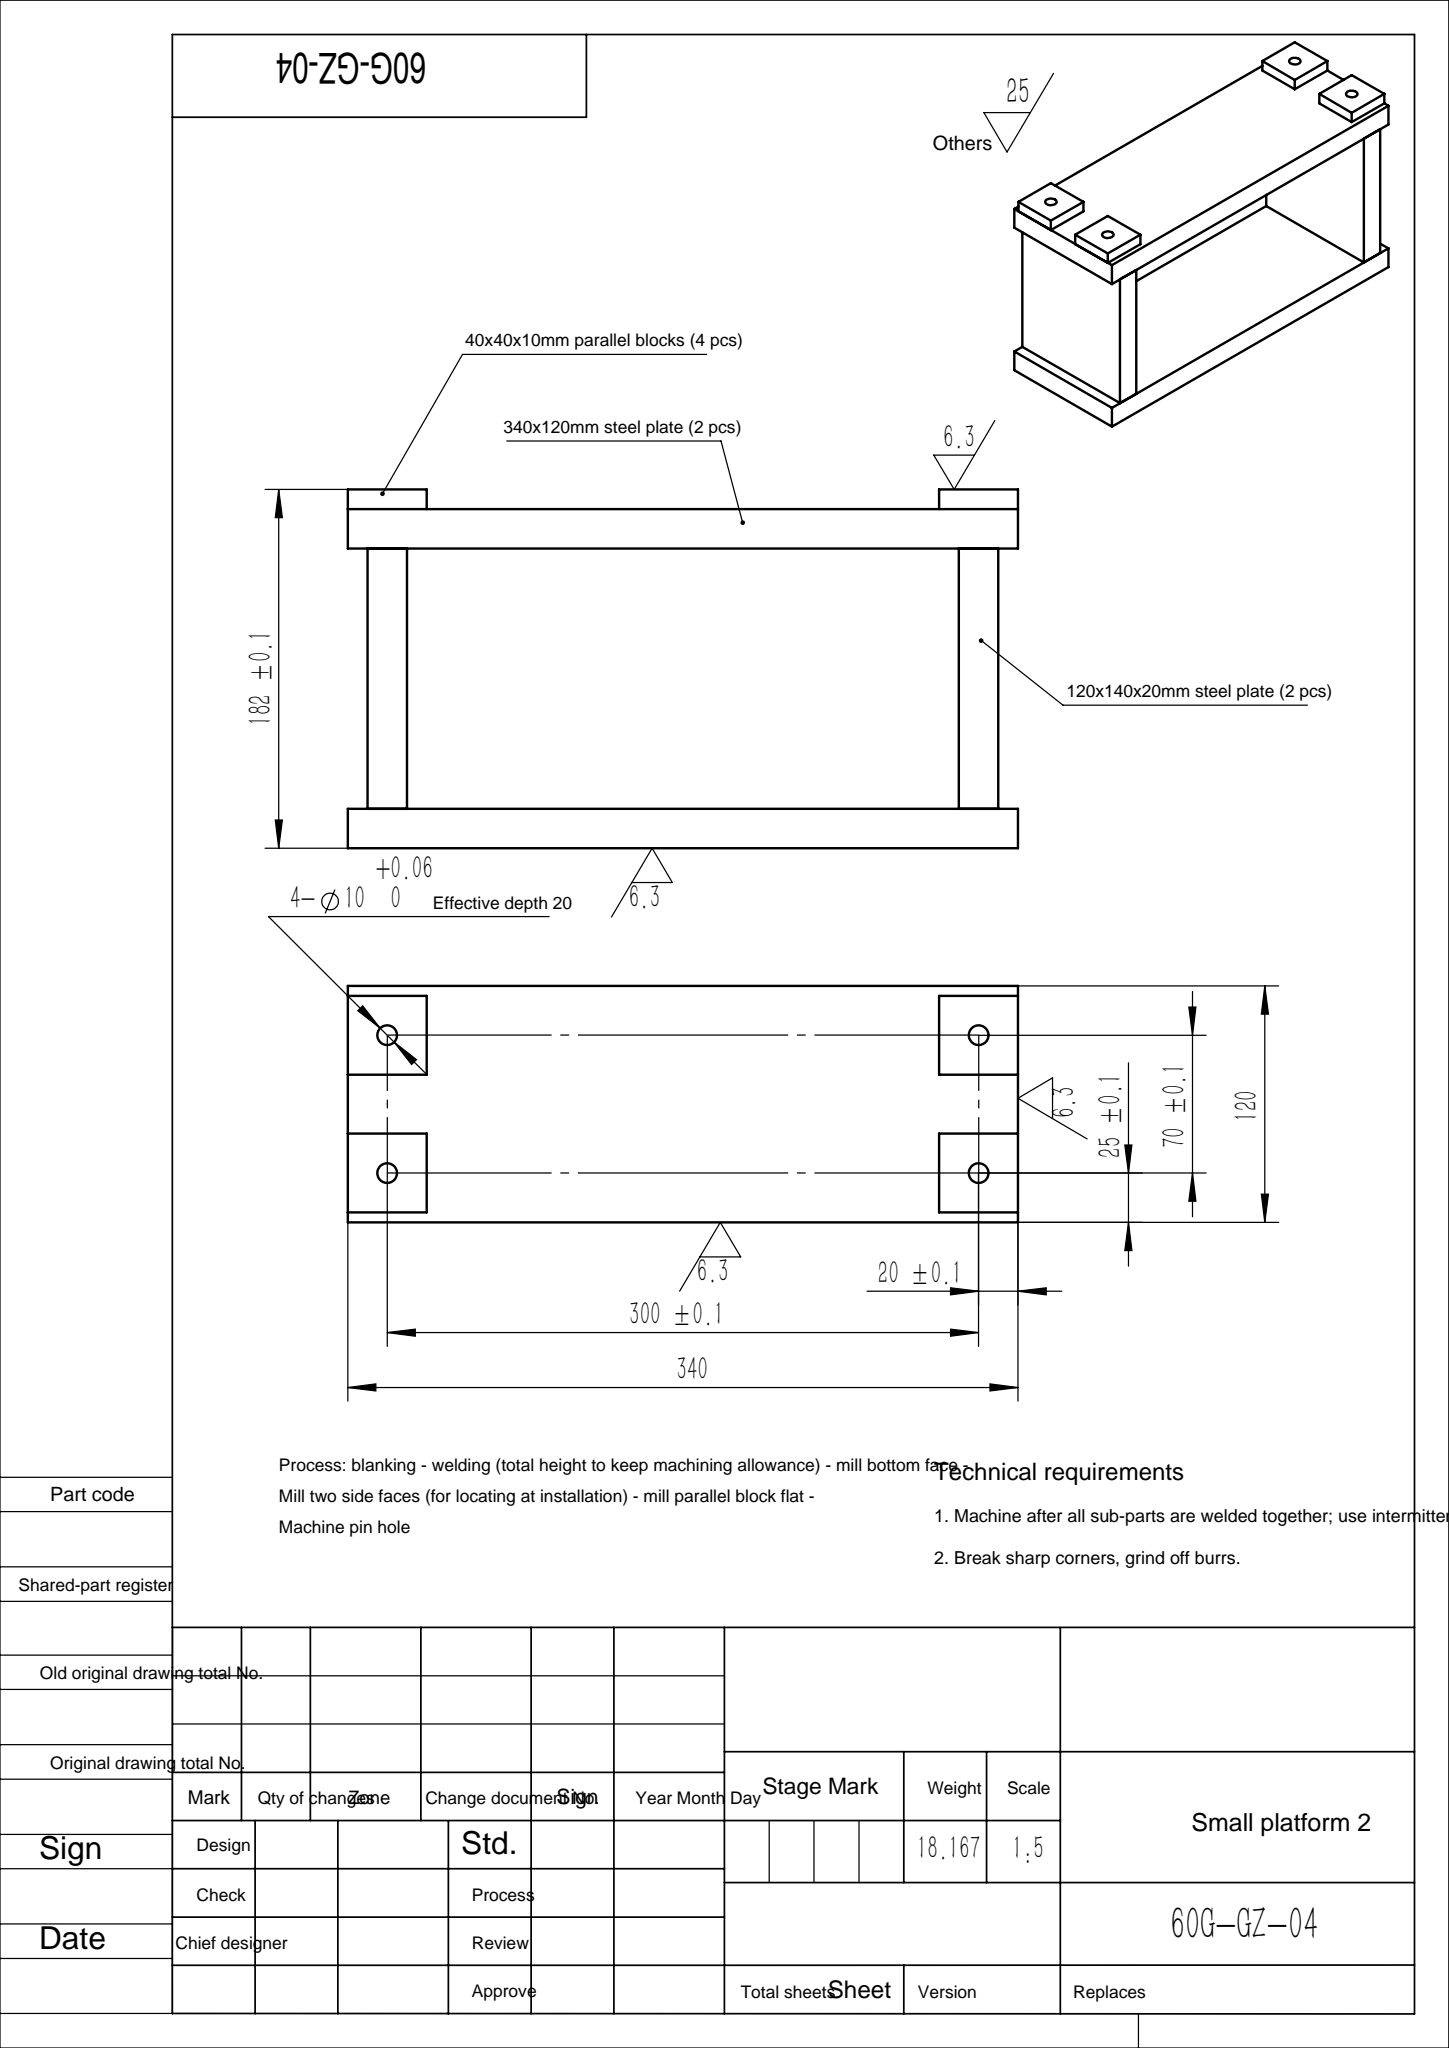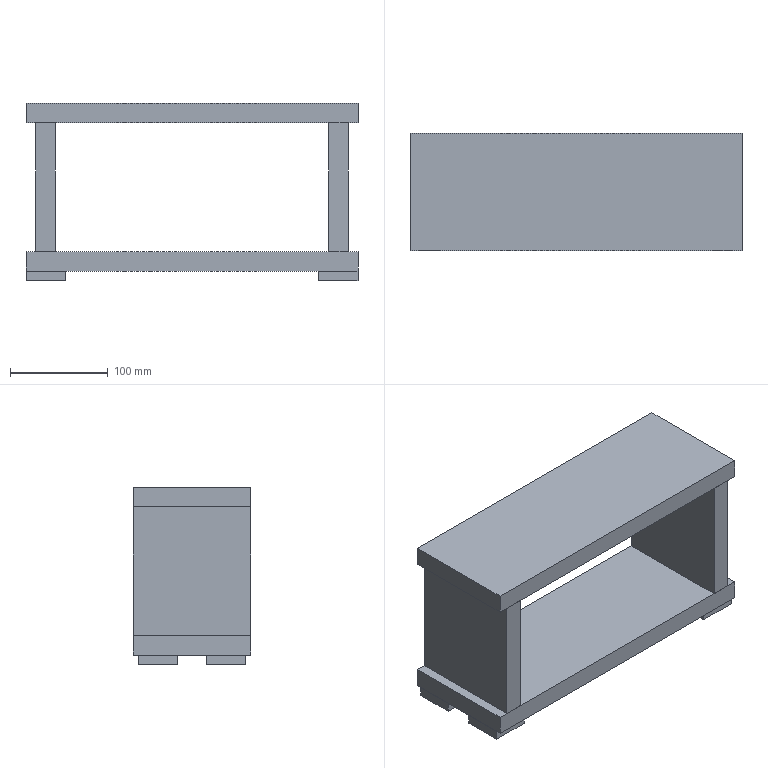Part | SolidWorks | features CompositeCurve 1 | 8 solids | 64 faces | box 340 x 120 x 182 mm | volume 2320175 mm3 | plane 48 | cylinder 16 | commonest cylinder face diameters 10 x16